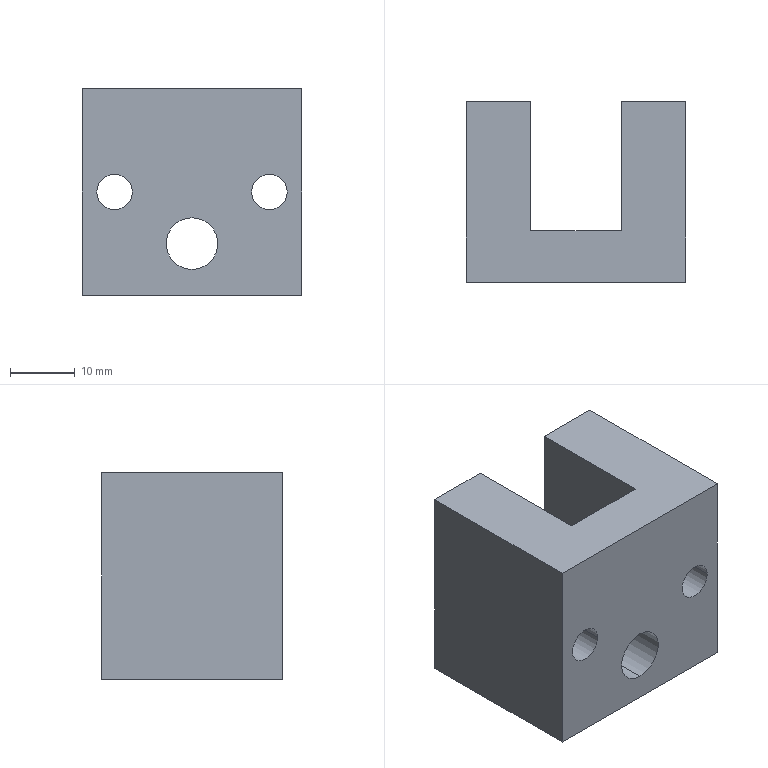Part | STEP file | push magnet slide seat | 1 solid | 30 faces | box 34 x 28 x 32 mm | volume 18978 mm3 | cylinder 14 | plane 12 | cone 4 | commonest cylinder face diameters 4.2 x4 5.5 x4 9 x4 8 x2